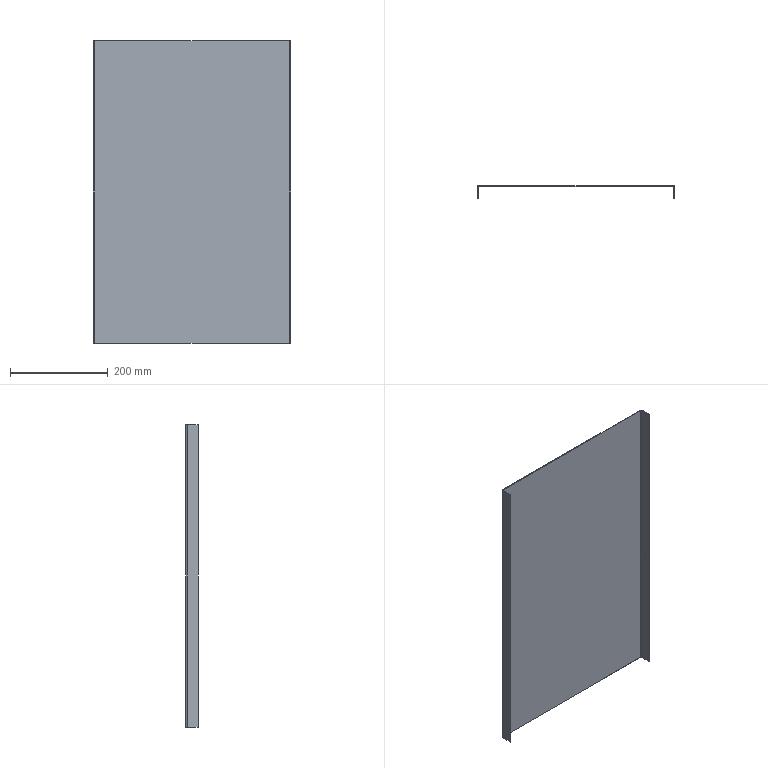Part | STEP file | ASND-0110-E63-HLTP01气SpringLower机架.4 | 1 solid | 14 faces | box 405 x 25 x 620 mm | volume 418564 mm3 | plane 10 | cylinder 4 | commonest cylinder face diameters 3 x2 6 x2
STEP:
#1=CARTESIAN_POINT('',(0.,0.,0.));
#2=DIRECTION('',(0.,0.,1.));
#3=DIRECTION('',(1.,0.,0.));
#4=AXIS2_PLACEMENT_3D('',#1,#2,#3);
#5=CARTESIAN_POINT('',(463.5,-3.,620.));
#6=VERTEX_POINT('',#5);
#7=CARTESIAN_POINT('',(463.5,-25.,620.));
#8=VERTEX_POINT('',#7);
#9=CARTESIAN_POINT('',(463.5,-3.,620.));
#10=DIRECTION('',(0.,-1.,0.));
#11=VECTOR('',#10,1.);
#12=LINE('',#9,#11);
#13=CARTESIAN_POINT('',(463.5,0.,1025.771));
#14=DIRECTION('',(1.,0.,0.));
#15=DIRECTION('',(0.,0.7071,0.7071));
#16=AXIS2_PLACEMENT_3D('',#13,#14,#15);
#17=PLANE('',#16);
#18=CARTESIAN_POINT('',(-289.045,-284.802));
#19=DIRECTION('',(-0.7071,0.7071));
#20=VECTOR('',#19,1.);
#21=LINE('',#18,#20);
#22=(GEOMETRIC_REPRESENTATION_CONTEXT(2)PARAMETRIC_REPRESENTATION_CONTEXT()REPRESENTATION_CONTEXT('',''));
#23=DEFINITIONAL_REPRESENTATION('',(#21),#22);
#24=PCURVE('',#17,#23);
#25=CARTESIAN_POINT('',(521.569,-40.,620.));
#26=DIRECTION('',(0.,0.,1.));
#27=DIRECTION('',(0.7071,0.7071,0.));
#28=AXIS2_PLACEMENT_3D('',#25,#26,#27);
#29=PLANE('',#28);
#30=CARTESIAN_POINT('',(-14.898,67.224));
#31=DIRECTION('',(-0.7071,-0.7071));
#32=VECTOR('',#31,1.);
#33=LINE('',#30,#32);
#34=(GEOMETRIC_REPRESENTATION_CONTEXT(2)PARAMETRIC_REPRESENTATION_CONTEXT()REPRESENTATION_CONTEXT('',''));
#35=DEFINITIONAL_REPRESENTATION('',(#33),#34);
#36=PCURVE('',#29,#35);
#37=SURFACE_CURVE('',#12,(#24,#36),.PCURVE_S1.);
#38=EDGE_CURVE('',#6,#8,#37,.T.);
#39=ORIENTED_EDGE('',*,*,#38,.F.);
#40=CARTESIAN_POINT('',(463.5,-3.,0.));
#41=VERTEX_POINT('',#40);
#42=CARTESIAN_POINT('',(463.5,-3.,620.));
#43=DIRECTION('',(0.,0.,-1.));
#44=VECTOR('',#43,1.);
#45=LINE('',#42,#44);
#46=CARTESIAN_POINT('',(-289.045,-284.802));
#47=DIRECTION('',(-0.7071,-0.7071));
#48=VECTOR('',#47,1.);
#49=LINE('',#46,#48);
#50=(GEOMETRIC_REPRESENTATION_CONTEXT(2)PARAMETRIC_REPRESENTATION_CONTEXT()REPRESENTATION_CONTEXT('',''));
#51=DEFINITIONAL_REPRESENTATION('',(#49),#50);
#52=PCURVE('',#17,#51);
#53=CARTESIAN_POINT('',(462.,-3.,1025.771));
#54=DIRECTION('',(0.,0.,1.));
#55=DIRECTION('',(1.,0.,0.));
#56=AXIS2_PLACEMENT_3D('',#53,#54,#55);
#57=CYLINDRICAL_SURFACE('',#56,1.5);
#58=CARTESIAN_POINT('',(0.,-405.771));
#59=DIRECTION('',(0.,-1.));
#60=VECTOR('',#59,1.);
#61=LINE('',#58,#60);
#62=(GEOMETRIC_REPRESENTATION_CONTEXT(2)PARAMETRIC_REPRESENTATION_CONTEXT()REPRESENTATION_CONTEXT('',''));
#63=DEFINITIONAL_REPRESENTATION('',(#61),#62);
#64=PCURVE('',#57,#63);
#65=SURFACE_CURVE('',#45,(#52,#64),.PCURVE_S1.);
#66=EDGE_CURVE('',#6,#41,#65,.T.);
#67=ORIENTED_EDGE('',*,*,#66,.T.);
#68=CARTESIAN_POINT('',(463.5,-25.,0.));
#69=VERTEX_POINT('',#68);
#70=CARTESIAN_POINT('',(463.5,-3.,0.));
#71=DIRECTION('',(0.,-1.,0.));
#72=VECTOR('',#71,1.);
#73=LINE('',#70,#72);
#74=CARTESIAN_POINT('',(-727.451,-723.208));
#75=DIRECTION('',(-0.7071,0.7071));
#76=VECTOR('',#75,1.);
#77=LINE('',#74,#76);
#78=(GEOMETRIC_REPRESENTATION_CONTEXT(2)PARAMETRIC_REPRESENTATION_CONTEXT()REPRESENTATION_CONTEXT('',''));
#79=DEFINITIONAL_REPRESENTATION('',(#77),#78);
#80=PCURVE('',#17,#79);
#81=CARTESIAN_POINT('',(0.,0.,0.));
#82=DIRECTION('',(0.,0.,-1.));
#83=DIRECTION('',(0.7071,0.7071,0.));
#84=AXIS2_PLACEMENT_3D('',#81,#82,#83);
#85=PLANE('',#84);
#86=CARTESIAN_POINT('',(325.623,329.865));
#87=DIRECTION('',(-0.7071,0.7071));
#88=VECTOR('',#87,1.);
#89=LINE('',#86,#88);
#90=(GEOMETRIC_REPRESENTATION_CONTEXT(2)PARAMETRIC_REPRESENTATION_CONTEXT()REPRESENTATION_CONTEXT('',''));
#91=DEFINITIONAL_REPRESENTATION('',(#89),#90);
#92=PCURVE('',#85,#91);
#93=SURFACE_CURVE('',#73,(#80,#92),.PCURVE_S1.);
#94=EDGE_CURVE('',#41,#69,#93,.T.);
#95=ORIENTED_EDGE('',*,*,#94,.T.);
#96=CARTESIAN_POINT('',(463.5,-25.,620.));
#97=DIRECTION('',(0.,0.,-1.));
#98=VECTOR('',#97,1.);
#99=LINE('',#96,#98);
#100=CARTESIAN_POINT('',(-304.601,-269.246));
#101=DIRECTION('',(-0.7071,-0.7071));
#102=VECTOR('',#101,1.);
#103=LINE('',#100,#102);
#104=(GEOMETRIC_REPRESENTATION_CONTEXT(2)PARAMETRIC_REPRESENTATION_CONTEXT()REPRESENTATION_CONTEXT('',''));
#105=DEFINITIONAL_REPRESENTATION('',(#103),#104);
#106=PCURVE('',#17,#105);
#107=CARTESIAN_POINT('',(465.,-25.,1025.771));
#108=DIRECTION('',(0.,-1.,0.));
#109=DIRECTION('',(0.7071,0.,0.7071));
#110=AXIS2_PLACEMENT_3D('',#107,#108,#109);
#111=PLANE('',#110);
#112=CARTESIAN_POINT('',(-287.984,-285.863));
#113=DIRECTION('',(-0.7071,-0.7071));
#114=VECTOR('',#113,1.);
#115=LINE('',#112,#114);
#116=(GEOMETRIC_REPRESENTATION_CONTEXT(2)PARAMETRIC_REPRESENTATION_CONTEXT()REPRESENTATION_CONTEXT('',''));
#117=DEFINITIONAL_REPRESENTATION('',(#115),#116);
#118=PCURVE('',#111,#117);
#119=SURFACE_CURVE('',#99,(#106,#118),.PCURVE_S1.);
#120=EDGE_CURVE('',#8,#69,#119,.T.);
#121=ORIENTED_EDGE('',*,*,#120,.F.);
#122=EDGE_LOOP('',(#39,#67,#95,#121));
#123=FACE_BOUND('',#122,.T.);
#124=ADVANCED_FACE('',(#123),#17,.F.);
#125=CARTESIAN_POINT('',(465.,-25.,620.));
#126=VERTEX_POINT('',#125);
#127=CARTESIAN_POINT('',(465.,-25.,0.));
#128=VERTEX_POINT('',#127);
#129=CARTESIAN_POINT('',(465.,-25.,620.));
#130=DIRECTION('',(0.,0.,-1.));
#131=VECTOR('',#130,1.);
#132=LINE('',#129,#131);
#133=CARTESIAN_POINT('',(-286.923,-286.923));
#134=DIRECTION('',(-0.7071,-0.7071));
#135=VECTOR('',#134,1.);
#136=LINE('',#133,#135);
#137=(GEOMETRIC_REPRESENTATION_CONTEXT(2)PARAMETRIC_REPRESENTATION_CONTEXT()REPRESENTATION_CONTEXT('',''));
#138=DEFINITIONAL_REPRESENTATION('',(#136),#137);
#139=PCURVE('',#111,#138);
#140=CARTESIAN_POINT('',(465.,0.,1025.771));
#141=DIRECTION('',(1.,0.,0.));
#142=DIRECTION('',(0.,0.7071,0.7071));
#143=AXIS2_PLACEMENT_3D('',#140,#141,#142);
#144=PLANE('',#143);
#145=CARTESIAN_POINT('',(-304.601,-269.246));
#146=DIRECTION('',(-0.7071,-0.7071));
#147=VECTOR('',#146,1.);
#148=LINE('',#145,#147);
#149=(GEOMETRIC_REPRESENTATION_CONTEXT(2)PARAMETRIC_REPRESENTATION_CONTEXT()REPRESENTATION_CONTEXT('',''));
#150=DEFINITIONAL_REPRESENTATION('',(#148),#149);
#151=PCURVE('',#144,#150);
#152=SURFACE_CURVE('',#132,(#139,#151),.PCURVE_S1.);
#153=EDGE_CURVE('',#126,#128,#152,.T.);
#154=ORIENTED_EDGE('',*,*,#153,.F.);
#155=CARTESIAN_POINT('',(465.,-25.,620.));
#156=DIRECTION('',(-1.,0.,0.));
#157=VECTOR('',#156,1.);
#158=LINE('',#155,#157);
#159=CARTESIAN_POINT('',(-286.923,-286.923));
#160=DIRECTION('',(-0.7071,0.7071));
#161=VECTOR('',#160,1.);
#162=LINE('',#159,#161);
#163=(GEOMETRIC_REPRESENTATION_CONTEXT(2)PARAMETRIC_REPRESENTATION_CONTEXT()REPRESENTATION_CONTEXT('',''));
#164=DEFINITIONAL_REPRESENTATION('',(#162),#163);
#165=PCURVE('',#111,#164);
#166=CARTESIAN_POINT('',(-29.393,50.607));
#167=DIRECTION('',(-0.7071,0.7071));
#168=VECTOR('',#167,1.);
#169=LINE('',#166,#168);
#170=(GEOMETRIC_REPRESENTATION_CONTEXT(2)PARAMETRIC_REPRESENTATION_CONTEXT()REPRESENTATION_CONTEXT('',''));
#171=DEFINITIONAL_REPRESENTATION('',(#169),#170);
#172=PCURVE('',#29,#171);
#173=SURFACE_CURVE('',#158,(#165,#172),.PCURVE_S1.);
#174=EDGE_CURVE('',#126,#8,#173,.T.);
#175=ORIENTED_EDGE('',*,*,#174,.T.);
#176=ORIENTED_EDGE('',*,*,#120,.T.);
#177=CARTESIAN_POINT('',(465.,-25.,0.));
#178=DIRECTION('',(-1.,0.,0.));
#179=VECTOR('',#178,1.);
#180=LINE('',#177,#179);
#181=CARTESIAN_POINT('',(-725.33,-725.33));
#182=DIRECTION('',(-0.7071,0.7071));
#183=VECTOR('',#182,1.);
#184=LINE('',#181,#183);
#185=(GEOMETRIC_REPRESENTATION_CONTEXT(2)PARAMETRIC_REPRESENTATION_CONTEXT()REPRESENTATION_CONTEXT('',''));
#186=DEFINITIONAL_REPRESENTATION('',(#184),#185);
#187=PCURVE('',#111,#186);
#188=CARTESIAN_POINT('',(311.127,346.482));
#189=DIRECTION('',(-0.7071,-0.7071));
#190=VECTOR('',#189,1.);
#191=LINE('',#188,#190);
#192=(GEOMETRIC_REPRESENTATION_CONTEXT(2)PARAMETRIC_REPRESENTATION_CONTEXT()REPRESENTATION_CONTEXT('',''));
#193=DEFINITIONAL_REPRESENTATION('',(#191),#192);
#194=PCURVE('',#85,#193);
#195=SURFACE_CURVE('',#180,(#187,#194),.PCURVE_S1.);
#196=EDGE_CURVE('',#128,#69,#195,.T.);
#197=ORIENTED_EDGE('',*,*,#196,.F.);
#198=EDGE_LOOP('',(#154,#175,#176,#197));
#199=FACE_BOUND('',#198,.T.);
#200=ADVANCED_FACE('',(#199),#111,.T.);
#201=CARTESIAN_POINT('',(465.,-3.,0.));
#202=VERTEX_POINT('',#201);
#203=CARTESIAN_POINT('',(465.,-3.,0.));
#204=DIRECTION('',(0.,-1.,0.));
#205=VECTOR('',#204,1.);
#206=LINE('',#203,#205);
#207=CARTESIAN_POINT('',(-727.451,-723.208));
#208=DIRECTION('',(-0.7071,0.7071));
#209=VECTOR('',#208,1.);
#210=LINE('',#207,#209);
#211=(GEOMETRIC_REPRESENTATION_CONTEXT(2)PARAMETRIC_REPRESENTATION_CONTEXT()REPRESENTATION_CONTEXT('',''));
#212=DEFINITIONAL_REPRESENTATION('',(#210),#211);
#213=PCURVE('',#144,#212);
#214=CARTESIAN_POINT('',(326.683,330.926));
#215=DIRECTION('',(-0.7071,0.7071));
#216=VECTOR('',#215,1.);
#217=LINE('',#214,#216);
#218=(GEOMETRIC_REPRESENTATION_CONTEXT(2)PARAMETRIC_REPRESENTATION_CONTEXT()REPRESENTATION_CONTEXT('',''));
#219=DEFINITIONAL_REPRESENTATION('',(#217),#218);
#220=PCURVE('',#85,#219);
#221=SURFACE_CURVE('',#206,(#213,#220),.PCURVE_S1.);
#222=EDGE_CURVE('',#202,#128,#221,.T.);
#223=ORIENTED_EDGE('',*,*,#222,.F.);
#224=CARTESIAN_POINT('',(465.,-3.,620.));
#225=VERTEX_POINT('',#224);
#226=CARTESIAN_POINT('',(465.,-3.,620.));
#227=DIRECTION('',(0.,0.,1.));
#228=VECTOR('',#227,1.);
#229=LINE('',#226,#228);
#230=CARTESIAN_POINT('',(-289.045,-284.802));
#231=DIRECTION('',(0.7071,0.7071));
#232=VECTOR('',#231,1.);
#233=LINE('',#230,#232);
#234=(GEOMETRIC_REPRESENTATION_CONTEXT(2)PARAMETRIC_REPRESENTATION_CONTEXT()REPRESENTATION_CONTEXT('',''));
#235=DEFINITIONAL_REPRESENTATION('',(#233),#234);
#236=PCURVE('',#144,#235);
#237=CARTESIAN_POINT('',(462.,-3.,1025.771));
#238=DIRECTION('',(0.,0.,-1.));
#239=DIRECTION('',(-1.,0.,0.));
#240=AXIS2_PLACEMENT_3D('',#237,#238,#239);
#241=CYLINDRICAL_SURFACE('',#240,3.);
#242=CARTESIAN_POINT('',(3.142,405.771));
#243=DIRECTION('',(0.,-1.));
#244=VECTOR('',#243,1.);
#245=LINE('',#242,#244);
#246=(GEOMETRIC_REPRESENTATION_CONTEXT(2)PARAMETRIC_REPRESENTATION_CONTEXT()REPRESENTATION_CONTEXT('',''));
#247=DEFINITIONAL_REPRESENTATION('',(#245),#246);
#248=PCURVE('',#241,#247);
#249=SURFACE_CURVE('',#229,(#236,#248),.PCURVE_S1.);
#250=EDGE_CURVE('',#202,#225,#249,.T.);
#251=ORIENTED_EDGE('',*,*,#250,.T.);
#252=CARTESIAN_POINT('',(465.,-3.,620.));
#253=DIRECTION('',(0.,-1.,0.));
#254=VECTOR('',#253,1.);
#255=LINE('',#252,#254);
#256=CARTESIAN_POINT('',(-289.045,-284.802));
#257=DIRECTION('',(-0.7071,0.7071));
#258=VECTOR('',#257,1.);
#259=LINE('',#256,#258);
#260=(GEOMETRIC_REPRESENTATION_CONTEXT(2)PARAMETRIC_REPRESENTATION_CONTEXT()REPRESENTATION_CONTEXT('',''));
#261=DEFINITIONAL_REPRESENTATION('',(#259),#260);
#262=PCURVE('',#144,#261);
#263=CARTESIAN_POINT('',(-13.837,66.163));
#264=DIRECTION('',(-0.7071,-0.7071));
#265=VECTOR('',#264,1.);
#266=LINE('',#263,#265);
#267=(GEOMETRIC_REPRESENTATION_CONTEXT(2)PARAMETRIC_REPRESENTATION_CONTEXT()REPRESENTATION_CONTEXT('',''));
#268=DEFINITIONAL_REPRESENTATION('',(#266),#267);
#269=PCURVE('',#29,#268);
#270=SURFACE_CURVE('',#255,(#262,#269),.PCURVE_S1.);
#271=EDGE_CURVE('',#225,#126,#270,.T.);
#272=ORIENTED_EDGE('',*,*,#271,.T.);
#273=ORIENTED_EDGE('',*,*,#153,.T.);
#274=EDGE_LOOP('',(#223,#251,#272,#273));
#275=FACE_BOUND('',#274,.T.);
#276=ADVANCED_FACE('',(#275),#144,.T.);
#277=CARTESIAN_POINT('',(63.,0.,620.));
#278=VERTEX_POINT('',#277);
#279=CARTESIAN_POINT('',(462.,0.,620.));
#280=VERTEX_POINT('',#279);
#281=CARTESIAN_POINT('',(63.,0.,620.));
#282=DIRECTION('',(1.,0.,0.));
#283=VECTOR('',#282,1.);
#284=LINE('',#281,#283);
#285=CARTESIAN_POINT('',(60.,0.,1025.771));
#286=DIRECTION('',(0.,1.,0.));
#287=DIRECTION('',(0.7071,0.,0.7071));
#288=AXIS2_PLACEMENT_3D('',#285,#286,#287);
#289=PLANE('',#288);
#290=CARTESIAN_POINT('',(-284.802,289.045));
#291=DIRECTION('',(0.7071,0.7071));
#292=VECTOR('',#291,1.);
#293=LINE('',#290,#292);
#294=(GEOMETRIC_REPRESENTATION_CONTEXT(2)PARAMETRIC_REPRESENTATION_CONTEXT()REPRESENTATION_CONTEXT('',''));
#295=DEFINITIONAL_REPRESENTATION('',(#293),#294);
#296=PCURVE('',#289,#295);
#297=CARTESIAN_POINT('',(-295.973,352.541));
#298=DIRECTION('',(0.7071,-0.7071));
#299=VECTOR('',#298,1.);
#300=LINE('',#297,#299);
#301=(GEOMETRIC_REPRESENTATION_CONTEXT(2)PARAMETRIC_REPRESENTATION_CONTEXT()REPRESENTATION_CONTEXT('',''));
#302=DEFINITIONAL_REPRESENTATION('',(#300),#301);
#303=PCURVE('',#29,#302);
#304=SURFACE_CURVE('',#284,(#296,#303),.PCURVE_S1.);
#305=EDGE_CURVE('',#278,#280,#304,.T.);
#306=ORIENTED_EDGE('',*,*,#305,.T.);
#307=CARTESIAN_POINT('',(462.,0.,0.));
#308=VERTEX_POINT('',#307);
#309=CARTESIAN_POINT('',(462.,0.,620.));
#310=DIRECTION('',(0.,0.,-1.));
#311=VECTOR('',#310,1.);
#312=LINE('',#309,#311);
#313=CARTESIAN_POINT('',(-2.666,571.18));
#314=DIRECTION('',(-0.7071,0.7071));
#315=VECTOR('',#314,1.);
#316=LINE('',#313,#315);
#317=(GEOMETRIC_REPRESENTATION_CONTEXT(2)PARAMETRIC_REPRESENTATION_CONTEXT()REPRESENTATION_CONTEXT('',''));
#318=DEFINITIONAL_REPRESENTATION('',(#316),#317);
#319=PCURVE('',#289,#318);
#320=CARTESIAN_POINT('',(1.571,405.771));
#321=DIRECTION('',(0.,1.));
#322=VECTOR('',#321,1.);
#323=LINE('',#320,#322);
#324=(GEOMETRIC_REPRESENTATION_CONTEXT(2)PARAMETRIC_REPRESENTATION_CONTEXT()REPRESENTATION_CONTEXT('',''));
#325=DEFINITIONAL_REPRESENTATION('',(#323),#324);
#326=PCURVE('',#241,#325);
#327=SURFACE_CURVE('',#312,(#319,#326),.PCURVE_S1.);
#328=EDGE_CURVE('',#280,#308,#327,.T.);
#329=ORIENTED_EDGE('',*,*,#328,.T.);
#330=CARTESIAN_POINT('',(63.,0.,0.));
#331=VERTEX_POINT('',#330);
#332=CARTESIAN_POINT('',(63.,0.,0.));
#333=DIRECTION('',(1.,0.,0.));
#334=VECTOR('',#333,1.);
#335=LINE('',#332,#334);
#336=CARTESIAN_POINT('',(-723.208,727.451));
#337=DIRECTION('',(0.7071,0.7071));
#338=VECTOR('',#337,1.);
#339=LINE('',#336,#338);
#340=(GEOMETRIC_REPRESENTATION_CONTEXT(2)PARAMETRIC_REPRESENTATION_CONTEXT()REPRESENTATION_CONTEXT('',''));
#341=DEFINITIONAL_REPRESENTATION('',(#339),#340);
#342=PCURVE('',#289,#341);
#343=CARTESIAN_POINT('',(44.548,44.548));
#344=DIRECTION('',(0.7071,0.7071));
#345=VECTOR('',#344,1.);
#346=LINE('',#343,#345);
#347=(GEOMETRIC_REPRESENTATION_CONTEXT(2)PARAMETRIC_REPRESENTATION_CONTEXT()REPRESENTATION_CONTEXT('',''));
#348=DEFINITIONAL_REPRESENTATION('',(#346),#347);
#349=PCURVE('',#85,#348);
#350=SURFACE_CURVE('',#335,(#342,#349),.PCURVE_S1.);
#351=EDGE_CURVE('',#331,#308,#350,.T.);
#352=ORIENTED_EDGE('',*,*,#351,.F.);
#353=CARTESIAN_POINT('',(63.,0.,620.));
#354=DIRECTION('',(0.,0.,1.));
#355=VECTOR('',#354,1.);
#356=LINE('',#353,#355);
#357=CARTESIAN_POINT('',(-284.802,289.045));
#358=DIRECTION('',(0.7071,-0.7071));
#359=VECTOR('',#358,1.);
#360=LINE('',#357,#359);
#361=(GEOMETRIC_REPRESENTATION_CONTEXT(2)PARAMETRIC_REPRESENTATION_CONTEXT()REPRESENTATION_CONTEXT('',''));
#362=DEFINITIONAL_REPRESENTATION('',(#360),#361);
#363=PCURVE('',#289,#362);
#364=CARTESIAN_POINT('',(63.,-3.,1025.771));
#365=DIRECTION('',(0.,0.,-1.));
#366=DIRECTION('',(-1.,0.,0.));
#367=AXIS2_PLACEMENT_3D('',#364,#365,#366);
#368=CYLINDRICAL_SURFACE('',#367,3.);
#369=CARTESIAN_POINT('',(1.571,405.771));
#370=DIRECTION('',(0.,-1.));
#371=VECTOR('',#370,1.);
#372=LINE('',#369,#371);
#373=(GEOMETRIC_REPRESENTATION_CONTEXT(2)PARAMETRIC_REPRESENTATION_CONTEXT()REPRESENTATION_CONTEXT('',''));
#374=DEFINITIONAL_REPRESENTATION('',(#372),#373);
#375=PCURVE('',#368,#374);
#376=SURFACE_CURVE('',#356,(#363,#375),.PCURVE_S1.);
#377=EDGE_CURVE('',#331,#278,#376,.T.);
#378=ORIENTED_EDGE('',*,*,#377,.T.);
#379=EDGE_LOOP('',(#306,#329,#352,#378));
#380=FACE_BOUND('',#379,.T.);
#381=ADVANCED_FACE('',(#380),#289,.T.);
#382=CARTESIAN_POINT('',(60.,-25.,620.));
#383=VERTEX_POINT('',#382);
#384=CARTESIAN_POINT('',(60.,-3.,620.));
#385=VERTEX_POINT('',#384);
#386=CARTESIAN_POINT('',(60.,-25.,620.));
#387=DIRECTION('',(0.,1.,0.));
#388=VECTOR('',#387,1.);
#389=LINE('',#386,#388);
#390=CARTESIAN_POINT('',(60.,-25.,1025.771));
#391=DIRECTION('',(-1.,0.,0.));
#392=DIRECTION('',(0.,0.7071,0.7071));
#393=AXIS2_PLACEMENT_3D('',#390,#391,#392);
#394=PLANE('',#393);
#395=CARTESIAN_POINT('',(-286.923,286.923));
#396=DIRECTION('',(0.7071,0.7071));
#397=VECTOR('',#396,1.);
#398=LINE('',#395,#397);
#399=(GEOMETRIC_REPRESENTATION_CONTEXT(2)PARAMETRIC_REPRESENTATION_CONTEXT()REPRESENTATION_CONTEXT('',''));
#400=DEFINITIONAL_REPRESENTATION('',(#398),#399);
#401=PCURVE('',#394,#400);
#402=CARTESIAN_POINT('',(-315.772,336.985));
#403=DIRECTION('',(0.7071,0.7071));
#404=VECTOR('',#403,1.);
#405=LINE('',#402,#404);
#406=(GEOMETRIC_REPRESENTATION_CONTEXT(2)PARAMETRIC_REPRESENTATION_CONTEXT()REPRESENTATION_CONTEXT('',''));
#407=DEFINITIONAL_REPRESENTATION('',(#405),#406);
#408=PCURVE('',#29,#407);
#409=SURFACE_CURVE('',#389,(#401,#408),.PCURVE_S1.);
#410=EDGE_CURVE('',#383,#385,#409,.T.);
#411=ORIENTED_EDGE('',*,*,#410,.T.);
#412=CARTESIAN_POINT('',(60.,-3.,0.));
#413=VERTEX_POINT('',#412);
#414=CARTESIAN_POINT('',(60.,-3.,620.));
#415=DIRECTION('',(0.,0.,-1.));
#416=VECTOR('',#415,1.);
#417=LINE('',#414,#416);
#418=CARTESIAN_POINT('',(-271.367,302.48));
#419=DIRECTION('',(-0.7071,0.7071));
#420=VECTOR('',#419,1.);
#421=LINE('',#418,#420);
#422=(GEOMETRIC_REPRESENTATION_CONTEXT(2)PARAMETRIC_REPRESENTATION_CONTEXT()REPRESENTATION_CONTEXT('',''));
#423=DEFINITIONAL_REPRESENTATION('',(#421),#422);
#424=PCURVE('',#394,#423);
#425=CARTESIAN_POINT('',(0.,405.771));
#426=DIRECTION('',(0.,1.));
#427=VECTOR('',#426,1.);
#428=LINE('',#425,#427);
#429=(GEOMETRIC_REPRESENTATION_CONTEXT(2)PARAMETRIC_REPRESENTATION_CONTEXT()REPRESENTATION_CONTEXT('',''));
#430=DEFINITIONAL_REPRESENTATION('',(#428),#429);
#431=PCURVE('',#368,#430);
#432=SURFACE_CURVE('',#417,(#424,#431),.PCURVE_S1.);
#433=EDGE_CURVE('',#385,#413,#432,.T.);
#434=ORIENTED_EDGE('',*,*,#433,.T.);
#435=CARTESIAN_POINT('',(60.,-25.,0.));
#436=VERTEX_POINT('',#435);
#437=CARTESIAN_POINT('',(60.,-25.,0.));
#438=DIRECTION('',(0.,1.,0.));
#439=VECTOR('',#438,1.);
#440=LINE('',#437,#439);
#441=CARTESIAN_POINT('',(-725.33,725.33));
#442=DIRECTION('',(0.7071,0.7071));
#443=VECTOR('',#442,1.);
#444=LINE('',#441,#443);
#445=(GEOMETRIC_REPRESENTATION_CONTEXT(2)PARAMETRIC_REPRESENTATION_CONTEXT()REPRESENTATION_CONTEXT('',''));
#446=DEFINITIONAL_REPRESENTATION('',(#444),#445);
#447=PCURVE('',#394,#446);
#448=CARTESIAN_POINT('',(24.749,60.104));
#449=DIRECTION('',(0.7071,-0.7071));
#450=VECTOR('',#449,1.);
#451=LINE('',#448,#450);
#452=(GEOMETRIC_REPRESENTATION_CONTEXT(2)PARAMETRIC_REPRESENTATION_CONTEXT()REPRESENTATION_CONTEXT('',''));
#453=DEFINITIONAL_REPRESENTATION('',(#451),#452);
#454=PCURVE('',#85,#453);
#455=SURFACE_CURVE('',#440,(#447,#454),.PCURVE_S1.);
#456=EDGE_CURVE('',#436,#413,#455,.T.);
#457=ORIENTED_EDGE('',*,*,#456,.F.);
#458=CARTESIAN_POINT('',(60.,-25.,620.));
#459=DIRECTION('',(0.,0.,-1.));
#460=VECTOR('',#459,1.);
#461=LINE('',#458,#460);
#462=CARTESIAN_POINT('',(-286.923,286.923));
#463=DIRECTION('',(-0.7071,0.7071));
#464=VECTOR('',#463,1.);
#465=LINE('',#462,#464);
#466=(GEOMETRIC_REPRESENTATION_CONTEXT(2)PARAMETRIC_REPRESENTATION_CONTEXT()REPRESENTATION_CONTEXT('',''));
#467=DEFINITIONAL_REPRESENTATION('',(#465),#466);
#468=PCURVE('',#394,#467);
#469=CARTESIAN_POINT('',(61.5,-25.,1025.771));
#470=DIRECTION('',(0.,-1.,0.));
#471=DIRECTION('',(0.7071,0.,0.7071));
#472=AXIS2_PLACEMENT_3D('',#469,#470,#471);
#473=PLANE('',#472);
#474=CARTESIAN_POINT('',(-287.984,-285.863));
#475=DIRECTION('',(-0.7071,-0.7071));
#476=VECTOR('',#475,1.);
#477=LINE('',#474,#476);
#478=(GEOMETRIC_REPRESENTATION_CONTEXT(2)PARAMETRIC_REPRESENTATION_CONTEXT()REPRESENTATION_CONTEXT('',''));
#479=DEFINITIONAL_REPRESENTATION('',(#477),#478);
#480=PCURVE('',#473,#479);
#481=SURFACE_CURVE('',#461,(#468,#480),.PCURVE_S1.);
#482=EDGE_CURVE('',#383,#436,#481,.T.);
#483=ORIENTED_EDGE('',*,*,#482,.F.);
#484=EDGE_LOOP('',(#411,#434,#457,#483));
#485=FACE_BOUND('',#484,.T.);
#486=ADVANCED_FACE('',(#485),#394,.T.);
#487=CARTESIAN_POINT('',(61.5,-25.,620.));
#488=VERTEX_POINT('',#487);
#489=CARTESIAN_POINT('',(61.5,-25.,0.));
#490=VERTEX_POINT('',#489);
#491=CARTESIAN_POINT('',(61.5,-25.,620.));
#492=DIRECTION('',(0.,0.,-1.));
#493=VECTOR('',#492,1.);
#494=LINE('',#491,#493);
#495=CARTESIAN_POINT('',(-286.923,-286.923));
#496=DIRECTION('',(-0.7071,-0.7071));
#497=VECTOR('',#496,1.);
#498=LINE('',#495,#497);
#499=(GEOMETRIC_REPRESENTATION_CONTEXT(2)PARAMETRIC_REPRESENTATION_CONTEXT()REPRESENTATION_CONTEXT('',''));
#500=DEFINITIONAL_REPRESENTATION('',(#498),#499);
#501=PCURVE('',#473,#500);
#502=CARTESIAN_POINT('',(61.5,-25.,1025.771));
#503=DIRECTION('',(-1.,0.,0.));
#504=DIRECTION('',(0.,0.7071,0.7071));
#505=AXIS2_PLACEMENT_3D('',#502,#503,#504);
#506=PLANE('',#505);
#507=CARTESIAN_POINT('',(-286.923,286.923));
#508=DIRECTION('',(-0.7071,0.7071));
#509=VECTOR('',#508,1.);
#510=LINE('',#507,#509);
#511=(GEOMETRIC_REPRESENTATION_CONTEXT(2)PARAMETRIC_REPRESENTATION_CONTEXT()REPRESENTATION_CONTEXT('',''));
#512=DEFINITIONAL_REPRESENTATION('',(#510),#511);
#513=PCURVE('',#506,#512);
#514=SURFACE_CURVE('',#494,(#501,#513),.PCURVE_S1.);
#515=EDGE_CURVE('',#488,#490,#514,.T.);
#516=ORIENTED_EDGE('',*,*,#515,.F.);
#517=CARTESIAN_POINT('',(61.5,-25.,620.));
#518=DIRECTION('',(-1.,0.,0.));
#519=VECTOR('',#518,1.);
#520=LINE('',#517,#519);
#521=CARTESIAN_POINT('',(-286.923,-286.923));
#522=DIRECTION('',(-0.7071,0.7071));
#523=VECTOR('',#522,1.);
#524=LINE('',#521,#523);
#525=(GEOMETRIC_REPRESENTATION_CONTEXT(2)PARAMETRIC_REPRESENTATION_CONTEXT()REPRESENTATION_CONTEXT('',''));
#526=DEFINITIONAL_REPRESENTATION('',(#524),#525);
#527=PCURVE('',#473,#526);
#528=CARTESIAN_POINT('',(-314.711,335.924));
#529=DIRECTION('',(-0.7071,0.7071));
#530=VECTOR('',#529,1.);
#531=LINE('',#528,#530);
#532=(GEOMETRIC_REPRESENTATION_CONTEXT(2)PARAMETRIC_REPRESENTATION_CONTEXT()REPRESENTATION_CONTEXT('',''));
#533=DEFINITIONAL_REPRESENTATION('',(#531),#532);
#534=PCURVE('',#29,#533);
#535=SURFACE_CURVE('',#520,(#527,#534),.PCURVE_S1.);
#536=EDGE_CURVE('',#488,#383,#535,.T.);
#537=ORIENTED_EDGE('',*,*,#536,.T.);
#538=ORIENTED_EDGE('',*,*,#482,.T.);
#539=CARTESIAN_POINT('',(61.5,-25.,0.));
#540=DIRECTION('',(-1.,0.,0.));
#541=VECTOR('',#540,1.);
#542=LINE('',#539,#541);
#543=CARTESIAN_POINT('',(-725.33,-725.33));
#544=DIRECTION('',(-0.7071,0.7071));
#545=VECTOR('',#544,1.);
#546=LINE('',#543,#545);
#547=(GEOMETRIC_REPRESENTATION_CONTEXT(2)PARAMETRIC_REPRESENTATION_CONTEXT()REPRESENTATION_CONTEXT('',''));
#548=DEFINITIONAL_REPRESENTATION('',(#546),#547);
#549=PCURVE('',#473,#548);
#550=CARTESIAN_POINT('',(25.809,61.165));
#551=DIRECTION('',(-0.7071,-0.7071));
#552=VECTOR('',#551,1.);
#553=LINE('',#550,#552);
#554=(GEOMETRIC_REPRESENTATION_CONTEXT(2)PARAMETRIC_REPRESENTATION_CONTEXT()REPRESENTATION_CONTEXT('',''));
#555=DEFINITIONAL_REPRESENTATION('',(#553),#554);
#556=PCURVE('',#85,#555);
#557=SURFACE_CURVE('',#542,(#549,#556),.PCURVE_S1.);
#558=EDGE_CURVE('',#490,#436,#557,.T.);
#559=ORIENTED_EDGE('',*,*,#558,.F.);
#560=EDGE_LOOP('',(#516,#537,#538,#559));
#561=FACE_BOUND('',#560,.T.);
#562=ADVANCED_FACE('',(#561),#473,.T.);
#563=CARTESIAN_POINT('',(61.5,-3.,0.));
#564=VERTEX_POINT('',#563);
#565=CARTESIAN_POINT('',(61.5,-25.,0.));
#566=DIRECTION('',(0.,1.,0.));
#567=VECTOR('',#566,1.);
#568=LINE('',#565,#567);
#569=CARTESIAN_POINT('',(-725.33,725.33));
#570=DIRECTION('',(0.7071,0.7071));
#571=VECTOR('',#570,1.);
#572=LINE('',#569,#571);
#573=(GEOMETRIC_REPRESENTATION_CONTEXT(2)PARAMETRIC_REPRESENTATION_CONTEXT()REPRESENTATION_CONTEXT('',''));
#574=DEFINITIONAL_REPRESENTATION('',(#572),#573);
#575=PCURVE('',#506,#574);
#576=CARTESIAN_POINT('',(25.809,61.165));
#577=DIRECTION('',(0.7071,-0.7071));
#578=VECTOR('',#577,1.);
#579=LINE('',#576,#578);
#580=(GEOMETRIC_REPRESENTATION_CONTEXT(2)PARAMETRIC_REPRESENTATION_CONTEXT()REPRESENTATION_CONTEXT('',''));
#581=DEFINITIONAL_REPRESENTATION('',(#579),#580);
#582=PCURVE('',#85,#581);
#583=SURFACE_CURVE('',#568,(#575,#582),.PCURVE_S1.);
#584=EDGE_CURVE('',#490,#564,#583,.T.);
#585=ORIENTED_EDGE('',*,*,#584,.T.);
#586=CARTESIAN_POINT('',(61.5,-3.,620.));
#587=VERTEX_POINT('',#586);
#588=CARTESIAN_POINT('',(61.5,-3.,620.));
#589=DIRECTION('',(0.,0.,1.));
#590=VECTOR('',#589,1.);
#591=LINE('',#588,#590);
#592=CARTESIAN_POINT('',(-271.367,302.48));
#593=DIRECTION('',(0.7071,-0.7071));
#594=VECTOR('',#593,1.);
#595=LINE('',#592,#594);
#596=(GEOMETRIC_REPRESENTATION_CONTEXT(2)PARAMETRIC_REPRESENTATION_CONTEXT()REPRESENTATION_CONTEXT('',''));
#597=DEFINITIONAL_REPRESENTATION('',(#595),#596);
#598=PCURVE('',#506,#597);
#599=CARTESIAN_POINT('',(63.,-3.,1025.771));
#600=DIRECTION('',(0.,0.,1.));
#601=DIRECTION('',(1.,0.,0.));
#602=AXIS2_PLACEMENT_3D('',#599,#600,#601);
#603=CYLINDRICAL_SURFACE('',#602,1.5);
#604=CARTESIAN_POINT('',(3.142,-405.771));
#605=DIRECTION('',(0.,1.));
#606=VECTOR('',#605,1.);
#607=LINE('',#604,#606);
#608=(GEOMETRIC_REPRESENTATION_CONTEXT(2)PARAMETRIC_REPRESENTATION_CONTEXT()REPRESENTATION_CONTEXT('',''));
#609=DEFINITIONAL_REPRESENTATION('',(#607),#608);
#610=PCURVE('',#603,#609);
#611=SURFACE_CURVE('',#591,(#598,#610),.PCURVE_S1.);
#612=EDGE_CURVE('',#564,#587,#611,.T.);
#613=ORIENTED_EDGE('',*,*,#612,.T.);
#614=CARTESIAN_POINT('',(61.5,-25.,620.));
#615=DIRECTION('',(0.,1.,0.));
#616=VECTOR('',#615,1.);
#617=LINE('',#614,#616);
#618=CARTESIAN_POINT('',(-286.923,286.923));
#619=DIRECTION('',(0.7071,0.7071));
#620=VECTOR('',#619,1.);
#621=LINE('',#618,#620);
#622=(GEOMETRIC_REPRESENTATION_CONTEXT(2)PARAMETRIC_REPRESENTATION_CONTEXT()REPRESENTATION_CONTEXT('',''));
#623=DEFINITIONAL_REPRESENTATION('',(#621),#622);
#624=PCURVE('',#506,#623);
#625=CARTESIAN_POINT('',(-314.711,335.924));
#626=DIRECTION('',(0.7071,0.7071));
#627=VECTOR('',#626,1.);
#628=LINE('',#625,#627);
#629=(GEOMETRIC_REPRESENTATION_CONTEXT(2)PARAMETRIC_REPRESENTATION_CONTEXT()REPRESENTATION_CONTEXT('',''));
#630=DEFINITIONAL_REPRESENTATION('',(#628),#629);
#631=PCURVE('',#29,#630);
#632=SURFACE_CURVE('',#617,(#624,#631),.PCURVE_S1.);
#633=EDGE_CURVE('',#488,#587,#632,.T.);
#634=ORIENTED_EDGE('',*,*,#633,.F.);
#635=ORIENTED_EDGE('',*,*,#515,.T.);
#636=EDGE_LOOP('',(#585,#613,#634,#635));
#637=FACE_BOUND('',#636,.T.);
#638=ADVANCED_FACE('',(#637),#506,.F.);
#639=CARTESIAN_POINT('',(63.,-1.5,620.));
#640=VERTEX_POINT('',#639);
#641=CARTESIAN_POINT('',(462.,-1.5,620.));
#642=VERTEX_POINT('',#641);
#643=CARTESIAN_POINT('',(63.,-1.5,620.));
#644=DIRECTION('',(1.,0.,0.));
#645=VECTOR('',#644,1.);
#646=LINE('',#643,#645);
#647=CARTESIAN_POINT('',(60.,-1.5,1025.771));
#648=DIRECTION('',(0.,1.,0.));
#649=DIRECTION('',(0.7071,0.,0.7071));
#650=AXIS2_PLACEMENT_3D('',#647,#648,#649);
#651=PLANE('',#650);
#652=CARTESIAN_POINT('',(-284.802,289.045));
#653=DIRECTION('',(0.7071,0.7071));
#654=VECTOR('',#653,1.);
#655=LINE('',#652,#654);
#656=(GEOMETRIC_REPRESENTATION_CONTEXT(2)PARAMETRIC_REPRESENTATION_CONTEXT()REPRESENTATION_CONTEXT('',''));
#657=DEFINITIONAL_REPRESENTATION('',(#655),#656);
#658=PCURVE('',#651,#657);
#659=CARTESIAN_POINT('',(-297.033,351.481));
#660=DIRECTION('',(0.7071,-0.7071));
#661=VECTOR('',#660,1.);
#662=LINE('',#659,#661);
#663=(GEOMETRIC_REPRESENTATION_CONTEXT(2)PARAMETRIC_REPRESENTATION_CONTEXT()REPRESENTATION_CONTEXT('',''));
#664=DEFINITIONAL_REPRESENTATION('',(#662),#663);
#665=PCURVE('',#29,#664);
#666=SURFACE_CURVE('',#646,(#658,#665),.PCURVE_S1.);
#667=EDGE_CURVE('',#640,#642,#666,.T.);
#668=ORIENTED_EDGE('',*,*,#667,.F.);
#669=CARTESIAN_POINT('',(63.,-1.5,0.));
#670=VERTEX_POINT('',#669);
#671=CARTESIAN_POINT('',(63.,-1.5,620.));
#672=DIRECTION('',(0.,0.,-1.));
#673=VECTOR('',#672,1.);
#674=LINE('',#671,#673);
#675=CARTESIAN_POINT('',(-284.802,289.045));
#676=DIRECTION('',(-0.7071,0.7071));
#677=VECTOR('',#676,1.);
#678=LINE('',#675,#677);
#679=(GEOMETRIC_REPRESENTATION_CONTEXT(2)PARAMETRIC_REPRESENTATION_CONTEXT()REPRESENTATION_CONTEXT('',''));
#680=DEFINITIONAL_REPRESENTATION('',(#678),#679);
#681=PCURVE('',#651,#680);
#682=CARTESIAN_POINT('',(1.571,-405.771));
#683=DIRECTION('',(0.,-1.));
#684=VECTOR('',#683,1.);
#685=LINE('',#682,#684);
#686=(GEOMETRIC_REPRESENTATION_CONTEXT(2)PARAMETRIC_REPRESENTATION_CONTEXT()REPRESENTATION_CONTEXT('',''));
#687=DEFINITIONAL_REPRESENTATION('',(#685),#686);
#688=PCURVE('',#603,#687);
#689=SURFACE_CURVE('',#674,(#681,#688),.PCURVE_S1.);
#690=EDGE_CURVE('',#640,#670,#689,.T.);
#691=ORIENTED_EDGE('',*,*,#690,.T.);
#692=CARTESIAN_POINT('',(462.,-1.5,0.));
#693=VERTEX_POINT('',#692);
#694=CARTESIAN_POINT('',(63.,-1.5,0.));
#695=DIRECTION('',(1.,0.,0.));
#696=VECTOR('',#695,1.);
#697=LINE('',#694,#696);
#698=CARTESIAN_POINT('',(-723.208,727.451));
#699=DIRECTION('',(0.7071,0.7071));
#700=VECTOR('',#699,1.);
#701=LINE('',#698,#700);
#702=(GEOMETRIC_REPRESENTATION_CONTEXT(2)PARAMETRIC_REPRESENTATION_CONTEXT()REPRESENTATION_CONTEXT('',''));
#703=DEFINITIONAL_REPRESENTATION('',(#701),#702);
#704=PCURVE('',#651,#703);
#705=CARTESIAN_POINT('',(43.487,45.608));
#706=DIRECTION('',(0.7071,0.7071));
#707=VECTOR('',#706,1.);
#708=LINE('',#705,#707);
#709=(GEOMETRIC_REPRESENTATION_CONTEXT(2)PARAMETRIC_REPRESENTATION_CONTEXT()REPRESENTATION_CONTEXT('',''));
#710=DEFINITIONAL_REPRESENTATION('',(#708),#709);
#711=PCURVE('',#85,#710);
#712=SURFACE_CURVE('',#697,(#704,#711),.PCURVE_S1.);
#713=EDGE_CURVE('',#670,#693,#712,.T.);
#714=ORIENTED_EDGE('',*,*,#713,.T.);
#715=CARTESIAN_POINT('',(462.,-1.5,620.));
#716=DIRECTION('',(0.,0.,1.));
#717=VECTOR('',#716,1.);
#718=LINE('',#715,#717);
#719=CARTESIAN_POINT('',(-2.666,571.18));
#720=DIRECTION('',(0.7071,-0.7071));
#721=VECTOR('',#720,1.);
#722=LINE('',#719,#721);
#723=(GEOMETRIC_REPRESENTATION_CONTEXT(2)PARAMETRIC_REPRESENTATION_CONTEXT()REPRESENTATION_CONTEXT('',''));
#724=DEFINITIONAL_REPRESENTATION('',(#722),#723);
#725=PCURVE('',#651,#724);
#726=CARTESIAN_POINT('',(1.571,-405.771));
#727=DIRECTION('',(0.,1.));
#728=VECTOR('',#727,1.);
#729=LINE('',#726,#728);
#730=(GEOMETRIC_REPRESENTATION_CONTEXT(2)PARAMETRIC_REPRESENTATION_CONTEXT()REPRESENTATION_CONTEXT('',''));
#731=DEFINITIONAL_REPRESENTATION('',(#729),#730);
#732=PCURVE('',#57,#731);
#733=SURFACE_CURVE('',#718,(#725,#732),.PCURVE_S1.);
#734=EDGE_CURVE('',#693,#642,#733,.T.);
#735=ORIENTED_EDGE('',*,*,#734,.T.);
#736=EDGE_LOOP('',(#668,#691,#714,#735));
#737=FACE_BOUND('',#736,.T.);
#738=ADVANCED_FACE('',(#737),#651,.F.);
#739=ORIENTED_EDGE('',*,*,#351,.T.);
#740=CARTESIAN_POINT('',(462.,-3.,0.));
#741=DIRECTION('',(0.,0.,-1.));
#742=DIRECTION('',(-1.,0.,0.));
#743=AXIS2_PLACEMENT_3D('',#740,#741,#742);
#744=CIRCLE('',#743,3.);
#745=CARTESIAN_POINT('',(324.562,328.805));
#746=DIRECTION('',(-0.7071,-0.7071));
#747=AXIS2_PLACEMENT_2D('',#745,#746);
#748=CIRCLE('',#747,3.);
#749=(GEOMETRIC_REPRESENTATION_CONTEXT(2)PARAMETRIC_REPRESENTATION_CONTEXT()REPRESENTATION_CONTEXT('',''));
#750=DEFINITIONAL_REPRESENTATION('',(#748),#749);
#751=PCURVE('',#85,#750);
#752=CARTESIAN_POINT('',(0.,1025.771));
#753=DIRECTION('',(1.,0.));
#754=VECTOR('',#753,1.);
#755=LINE('',#752,#754);
#756=(GEOMETRIC_REPRESENTATION_CONTEXT(2)PARAMETRIC_REPRESENTATION_CONTEXT()REPRESENTATION_CONTEXT('',''));
#757=DEFINITIONAL_REPRESENTATION('',(#755),#756);
#758=PCURVE('',#241,#757);
#759=SURFACE_CURVE('',#744,(#751,#758),.PCURVE_S1.);
#760=EDGE_CURVE('',#308,#202,#759,.T.);
#761=ORIENTED_EDGE('',*,*,#760,.T.);
#762=ORIENTED_EDGE('',*,*,#222,.T.);
#763=ORIENTED_EDGE('',*,*,#196,.T.);
#764=ORIENTED_EDGE('',*,*,#94,.F.);
#765=CARTESIAN_POINT('',(462.,-3.,0.));
#766=DIRECTION('',(0.,0.,1.));
#767=DIRECTION('',(-1.,0.,0.));
#768=AXIS2_PLACEMENT_3D('',#765,#766,#767);
#769=CIRCLE('',#768,1.5);
#770=CARTESIAN_POINT('',(323.501,327.744));
#771=CARTESIAN_POINT('',(321.664,329.581));
#772=CARTESIAN_POINT('',(324.174,330.254));
#773=CARTESIAN_POINT('',(326.683,330.926));
#774=CARTESIAN_POINT('',(326.011,328.416));
#775=CARTESIAN_POINT('',(325.338,325.907));
#776=CARTESIAN_POINT('',(323.501,327.744));
#777=(BOUNDED_CURVE()B_SPLINE_CURVE(2,(#770,#771,#772,#773,#774,#775,#776),.UNSPECIFIED.,.T.,.F.)B_SPLINE_CURVE_WITH_KNOTS((1,2,2,2,2,1),(-2.094,0.,2.094,4.189,6.283,8.378),.UNSPECIFIED.)CURVE()GEOMETRIC_REPRESENTATION_ITEM()RATIONAL_B_SPLINE_CURVE((1.,0.5,1.,0.5,1.,0.5,1.))REPRESENTATION_ITEM(''));
#778=(GEOMETRIC_REPRESENTATION_CONTEXT(2)PARAMETRIC_REPRESENTATION_CONTEXT()REPRESENTATION_CONTEXT('',''));
#779=DEFINITIONAL_REPRESENTATION('',(#777),#778);
#780=PCURVE('',#85,#779);
#781=CARTESIAN_POINT('',(-3.142,-1025.771));
#782=DIRECTION('',(1.,0.));
#783=VECTOR('',#782,1.);
#784=LINE('',#781,#783);
#785=(GEOMETRIC_REPRESENTATION_CONTEXT(2)PARAMETRIC_REPRESENTATION_CONTEXT()REPRESENTATION_CONTEXT('',''));
#786=DEFINITIONAL_REPRESENTATION('',(#784),#785);
#787=PCURVE('',#57,#786);
#788=SURFACE_CURVE('',#769,(#780,#787),.PCURVE_S1.);
#789=EDGE_CURVE('',#41,#693,#788,.T.);
#790=ORIENTED_EDGE('',*,*,#789,.T.);
#791=ORIENTED_EDGE('',*,*,#713,.F.);
#792=CARTESIAN_POINT('',(63.,-3.,0.));
#793=DIRECTION('',(0.,0.,1.));
#794=DIRECTION('',(-1.,0.,0.));
#795=AXIS2_PLACEMENT_3D('',#792,#793,#794);
#796=CIRCLE('',#795,1.5);
#797=CARTESIAN_POINT('',(41.366,45.608));
#798=CARTESIAN_POINT('',(39.529,47.446));
#799=CARTESIAN_POINT('',(42.038,48.118));
#800=CARTESIAN_POINT('',(44.548,48.79));
#801=CARTESIAN_POINT('',(43.875,46.281));
#802=CARTESIAN_POINT('',(43.203,43.771));
#803=CARTESIAN_POINT('',(41.366,45.608));
#804=(BOUNDED_CURVE()B_SPLINE_CURVE(2,(#797,#798,#799,#800,#801,#802,#803),.UNSPECIFIED.,.T.,.F.)B_SPLINE_CURVE_WITH_KNOTS((1,2,2,2,2,1),(-2.094,0.,2.094,4.189,6.283,8.378),.UNSPECIFIED.)CURVE()GEOMETRIC_REPRESENTATION_ITEM()RATIONAL_B_SPLINE_CURVE((1.,0.5,1.,0.5,1.,0.5,1.))REPRESENTATION_ITEM(''));
#805=(GEOMETRIC_REPRESENTATION_CONTEXT(2)PARAMETRIC_REPRESENTATION_CONTEXT()REPRESENTATION_CONTEXT('',''));
#806=DEFINITIONAL_REPRESENTATION('',(#804),#805);
#807=PCURVE('',#85,#806);
#808=CARTESIAN_POINT('',(-3.142,-1025.771));
#809=DIRECTION('',(1.,0.));
#810=VECTOR('',#809,1.);
#811=LINE('',#808,#810);
#812=(GEOMETRIC_REPRESENTATION_CONTEXT(2)PARAMETRIC_REPRESENTATION_CONTEXT()REPRESENTATION_CONTEXT('',''));
#813=DEFINITIONAL_REPRESENTATION('',(#811),#812);
#814=PCURVE('',#603,#813);
#815=SURFACE_CURVE('',#796,(#807,#814),.PCURVE_S1.);
#816=EDGE_CURVE('',#670,#564,#815,.T.);
#817=ORIENTED_EDGE('',*,*,#816,.T.);
#818=ORIENTED_EDGE('',*,*,#584,.F.);
#819=ORIENTED_EDGE('',*,*,#558,.T.);
#820=ORIENTED_EDGE('',*,*,#456,.T.);
#821=CARTESIAN_POINT('',(63.,-3.,0.));
#822=DIRECTION('',(0.,0.,-1.));
#823=DIRECTION('',(-1.,0.,0.));
#824=AXIS2_PLACEMENT_3D('',#821,#822,#823);
#825=CIRCLE('',#824,3.);
#826=CARTESIAN_POINT('',(42.426,46.669));
#827=DIRECTION('',(-0.7071,-0.7071));
#828=AXIS2_PLACEMENT_2D('',#826,#827);
#829=CIRCLE('',#828,3.);
#830=(GEOMETRIC_REPRESENTATION_CONTEXT(2)PARAMETRIC_REPRESENTATION_CONTEXT()REPRESENTATION_CONTEXT('',''));
#831=DEFINITIONAL_REPRESENTATION('',(#829),#830);
#832=PCURVE('',#85,#831);
#833=CARTESIAN_POINT('',(0.,1025.771));
#834=DIRECTION('',(1.,0.));
#835=VECTOR('',#834,1.);
#836=LINE('',#833,#835);
#837=(GEOMETRIC_REPRESENTATION_CONTEXT(2)PARAMETRIC_REPRESENTATION_CONTEXT()REPRESENTATION_CONTEXT('',''));
#838=DEFINITIONAL_REPRESENTATION('',(#836),#837);
#839=PCURVE('',#368,#838);
#840=SURFACE_CURVE('',#825,(#832,#839),.PCURVE_S1.);
#841=EDGE_CURVE('',#413,#331,#840,.T.);
#842=ORIENTED_EDGE('',*,*,#841,.T.);
#843=EDGE_LOOP('',(#739,#761,#762,#763,#764,#790,#791,#817,#818,#819,#820,#842));
#844=FACE_BOUND('',#843,.T.);
#845=ADVANCED_FACE('',(#844),#85,.T.);
#846=ORIENTED_EDGE('',*,*,#271,.F.);
#847=CARTESIAN_POINT('',(462.,-3.,620.));
#848=DIRECTION('',(0.,0.,1.));
#849=DIRECTION('',(1.,0.,0.));
#850=AXIS2_PLACEMENT_3D('',#847,#848,#849);
#851=CIRCLE('',#850,3.);
#852=CARTESIAN_POINT('',(-15.958,68.284));
#853=DIRECTION('',(0.7071,-0.7071));
#854=AXIS2_PLACEMENT_2D('',#852,#853);
#855=CIRCLE('',#854,3.);
#856=(GEOMETRIC_REPRESENTATION_CONTEXT(2)PARAMETRIC_REPRESENTATION_CONTEXT()REPRESENTATION_CONTEXT('',''));
#857=DEFINITIONAL_REPRESENTATION('',(#855),#856);
#858=PCURVE('',#29,#857);
#859=CARTESIAN_POINT('',(3.142,405.771));
#860=DIRECTION('',(-1.,0.));
#861=VECTOR('',#860,1.);
#862=LINE('',#859,#861);
#863=(GEOMETRIC_REPRESENTATION_CONTEXT(2)PARAMETRIC_REPRESENTATION_CONTEXT()REPRESENTATION_CONTEXT('',''));
#864=DEFINITIONAL_REPRESENTATION('',(#862),#863);
#865=PCURVE('',#241,#864);
#866=SURFACE_CURVE('',#851,(#858,#865),.PCURVE_S1.);
#867=EDGE_CURVE('',#225,#280,#866,.T.);
#868=ORIENTED_EDGE('',*,*,#867,.T.);
#869=ORIENTED_EDGE('',*,*,#305,.F.);
#870=CARTESIAN_POINT('',(63.,-3.,620.));
#871=DIRECTION('',(0.,0.,1.));
#872=DIRECTION('',(1.,0.,0.));
#873=AXIS2_PLACEMENT_3D('',#870,#871,#872);
#874=CIRCLE('',#873,3.);
#875=CARTESIAN_POINT('',(-298.094,350.42));
#876=DIRECTION('',(0.7071,-0.7071));
#877=AXIS2_PLACEMENT_2D('',#875,#876);
#878=CIRCLE('',#877,3.);
#879=(GEOMETRIC_REPRESENTATION_CONTEXT(2)PARAMETRIC_REPRESENTATION_CONTEXT()REPRESENTATION_CONTEXT('',''));
#880=DEFINITIONAL_REPRESENTATION('',(#878),#879);
#881=PCURVE('',#29,#880);
#882=CARTESIAN_POINT('',(3.142,405.771));
#883=DIRECTION('',(-1.,0.));
#884=VECTOR('',#883,1.);
#885=LINE('',#882,#884);
#886=(GEOMETRIC_REPRESENTATION_CONTEXT(2)PARAMETRIC_REPRESENTATION_CONTEXT()REPRESENTATION_CONTEXT('',''));
#887=DEFINITIONAL_REPRESENTATION('',(#885),#886);
#888=PCURVE('',#368,#887);
#889=SURFACE_CURVE('',#874,(#881,#888),.PCURVE_S1.);
#890=EDGE_CURVE('',#278,#385,#889,.T.);
#891=ORIENTED_EDGE('',*,*,#890,.T.);
#892=ORIENTED_EDGE('',*,*,#410,.F.);
#893=ORIENTED_EDGE('',*,*,#536,.F.);
#894=ORIENTED_EDGE('',*,*,#633,.T.);
#895=CARTESIAN_POINT('',(63.,-3.,620.));
#896=DIRECTION('',(0.,0.,-1.));
#897=DIRECTION('',(1.,0.,0.));
#898=AXIS2_PLACEMENT_3D('',#895,#896,#897);
#899=CIRCLE('',#898,1.5);
#900=CARTESIAN_POINT('',(-297.033,349.359));
#901=CARTESIAN_POINT('',(-298.87,347.522));
#902=CARTESIAN_POINT('',(-299.543,350.032));
#903=CARTESIAN_POINT('',(-300.215,352.541));
#904=CARTESIAN_POINT('',(-297.706,351.869));
#905=CARTESIAN_POINT('',(-295.196,351.196));
#906=CARTESIAN_POINT('',(-297.033,349.359));
#907=(BOUNDED_CURVE()B_SPLINE_CURVE(2,(#900,#901,#902,#903,#904,#905,#906),.UNSPECIFIED.,.T.,.F.)B_SPLINE_CURVE_WITH_KNOTS((1,2,2,2,2,1),(-2.094,0.,2.094,4.189,6.283,8.378),.UNSPECIFIED.)CURVE()GEOMETRIC_REPRESENTATION_ITEM()RATIONAL_B_SPLINE_CURVE((1.,0.5,1.,0.5,1.,0.5,1.))REPRESENTATION_ITEM(''));
#908=(GEOMETRIC_REPRESENTATION_CONTEXT(2)PARAMETRIC_REPRESENTATION_CONTEXT()REPRESENTATION_CONTEXT('',''));
#909=DEFINITIONAL_REPRESENTATION('',(#907),#908);
#910=PCURVE('',#29,#909);
#911=CARTESIAN_POINT('',(6.283,-405.771));
#912=DIRECTION('',(-1.,0.));
#913=VECTOR('',#912,1.);
#914=LINE('',#911,#913);
#915=(GEOMETRIC_REPRESENTATION_CONTEXT(2)PARAMETRIC_REPRESENTATION_CONTEXT()REPRESENTATION_CONTEXT('',''));
#916=DEFINITIONAL_REPRESENTATION('',(#914),#915);
#917=PCURVE('',#603,#916);
#918=SURFACE_CURVE('',#899,(#910,#917),.PCURVE_S1.);
#919=EDGE_CURVE('',#587,#640,#918,.T.);
#920=ORIENTED_EDGE('',*,*,#919,.T.);
#921=ORIENTED_EDGE('',*,*,#667,.T.);
#922=CARTESIAN_POINT('',(462.,-3.,620.));
#923=DIRECTION('',(0.,0.,-1.));
#924=DIRECTION('',(1.,0.,0.));
#925=AXIS2_PLACEMENT_3D('',#922,#923,#924);
#926=CIRCLE('',#925,1.5);
#927=CARTESIAN_POINT('',(-14.898,67.224));
#928=CARTESIAN_POINT('',(-16.735,65.386));
#929=CARTESIAN_POINT('',(-17.407,67.896));
#930=CARTESIAN_POINT('',(-18.08,70.406));
#931=CARTESIAN_POINT('',(-15.57,69.733));
#932=CARTESIAN_POINT('',(-13.061,69.061));
#933=CARTESIAN_POINT('',(-14.898,67.224));
#934=(BOUNDED_CURVE()B_SPLINE_CURVE(2,(#927,#928,#929,#930,#931,#932,#933),.UNSPECIFIED.,.T.,.F.)B_SPLINE_CURVE_WITH_KNOTS((1,2,2,2,2,1),(-2.094,0.,2.094,4.189,6.283,8.378),.UNSPECIFIED.)CURVE()GEOMETRIC_REPRESENTATION_ITEM()RATIONAL_B_SPLINE_CURVE((1.,0.5,1.,0.5,1.,0.5,1.))REPRESENTATION_ITEM(''));
#935=(GEOMETRIC_REPRESENTATION_CONTEXT(2)PARAMETRIC_REPRESENTATION_CONTEXT()REPRESENTATION_CONTEXT('',''));
#936=DEFINITIONAL_REPRESENTATION('',(#934),#935);
#937=PCURVE('',#29,#936);
#938=CARTESIAN_POINT('',(6.283,-405.771));
#939=DIRECTION('',(-1.,0.));
#940=VECTOR('',#939,1.);
#941=LINE('',#938,#940);
#942=(GEOMETRIC_REPRESENTATION_CONTEXT(2)PARAMETRIC_REPRESENTATION_CONTEXT()REPRESENTATION_CONTEXT('',''));
#943=DEFINITIONAL_REPRESENTATION('',(#941),#942);
#944=PCURVE('',#57,#943);
#945=SURFACE_CURVE('',#926,(#937,#944),.PCURVE_S1.);
#946=EDGE_CURVE('',#642,#6,#945,.T.);
#947=ORIENTED_EDGE('',*,*,#946,.T.);
#948=ORIENTED_EDGE('',*,*,#38,.T.);
#949=ORIENTED_EDGE('',*,*,#174,.F.);
#950=EDGE_LOOP('',(#846,#868,#869,#891,#892,#893,#894,#920,#921,#947,#948,#949));
#951=FACE_BOUND('',#950,.T.);
#952=ADVANCED_FACE('',(#951),#29,.T.);
#953=ORIENTED_EDGE('',*,*,#867,.F.);
#954=ORIENTED_EDGE('',*,*,#250,.F.);
#955=ORIENTED_EDGE('',*,*,#760,.F.);
#956=ORIENTED_EDGE('',*,*,#328,.F.);
#957=EDGE_LOOP('',(#953,#954,#955,#956));
#958=FACE_BOUND('',#957,.T.);
#959=ADVANCED_FACE('',(#958),#241,.T.);
#960=ORIENTED_EDGE('',*,*,#890,.F.);
#961=ORIENTED_EDGE('',*,*,#377,.F.);
#962=ORIENTED_EDGE('',*,*,#841,.F.);
#963=ORIENTED_EDGE('',*,*,#433,.F.);
#964=EDGE_LOOP('',(#960,#961,#962,#963));
#965=FACE_BOUND('',#964,.T.);
#966=ADVANCED_FACE('',(#965),#368,.T.);
#967=ORIENTED_EDGE('',*,*,#690,.T.);
#968=ORIENTED_EDGE('',*,*,#816,.T.);
#969=ORIENTED_EDGE('',*,*,#612,.T.);
#970=ORIENTED_EDGE('',*,*,#919,.T.);
#971=EDGE_LOOP('',(#967,#968,#969,#970));
#972=FACE_BOUND('',#971,.F.);
#973=ADVANCED_FACE('',(#972),#603,.F.);
#974=ORIENTED_EDGE('',*,*,#66,.T.);
#975=ORIENTED_EDGE('',*,*,#789,.T.);
#976=ORIENTED_EDGE('',*,*,#734,.T.);
#977=ORIENTED_EDGE('',*,*,#946,.T.);
#978=EDGE_LOOP('',(#974,#975,#976,#977));
#979=FACE_BOUND('',#978,.F.);
#980=ADVANCED_FACE('',(#979),#57,.F.);
#981=CLOSED_SHELL('',(#124,#200,#276,#381,#486,#562,#638,#738,#845,#952,#959,#966,#973,#980));
#982=MANIFOLD_SOLID_BREP('',#981);
#983=(LENGTH_UNIT()NAMED_UNIT(*)SI_UNIT(.MILLI.,.METRE.));
#984=UNCERTAINTY_MEASURE_WITH_UNIT(LENGTH_MEASURE(0.0000001),#983,'','');
#985=(NAMED_UNIT(*)PLANE_ANGLE_UNIT()SI_UNIT($,.RADIAN.));
#986=(NAMED_UNIT(*)SI_UNIT($,.STERADIAN.)SOLID_ANGLE_UNIT());
#987=(GEOMETRIC_REPRESENTATION_CONTEXT(3)GLOBAL_UNCERTAINTY_ASSIGNED_CONTEXT((#984))GLOBAL_UNIT_ASSIGNED_CONTEXT((#983,#985,#986))REPRESENTATION_CONTEXT('',''));
#988=ADVANCED_BREP_SHAPE_REPRESENTATION('',(#4,#982),#987);